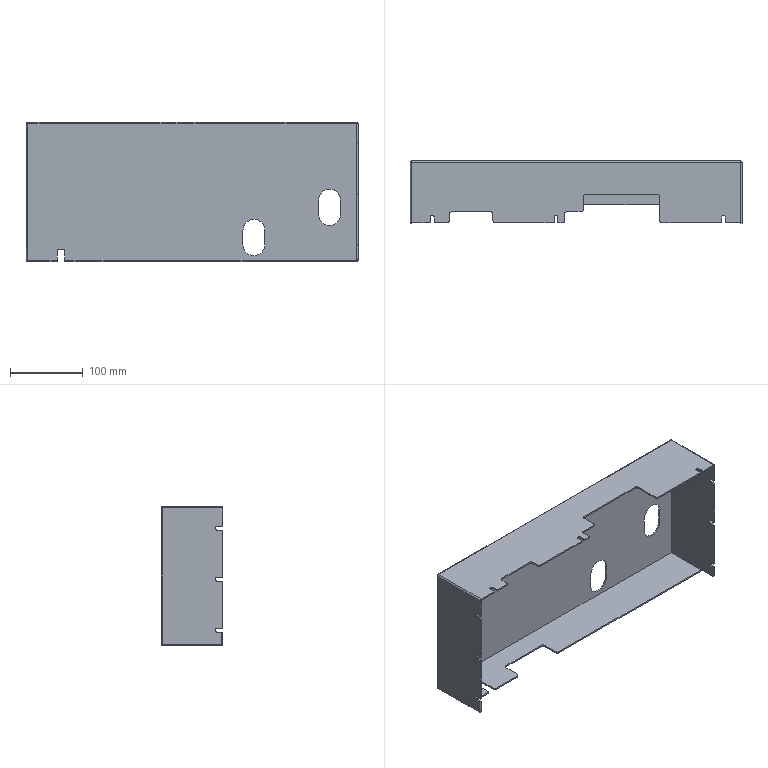Part | NX | features BREP 1 | 1 solid | 109 faces | box 456 x 85 x 191 mm | volume 341001 mm3 | plane 63 | cylinder 41 | sphere 4 | torus 1 | commonest cylinder face diameters 6 x16 4 x10 5 x9 30 x6